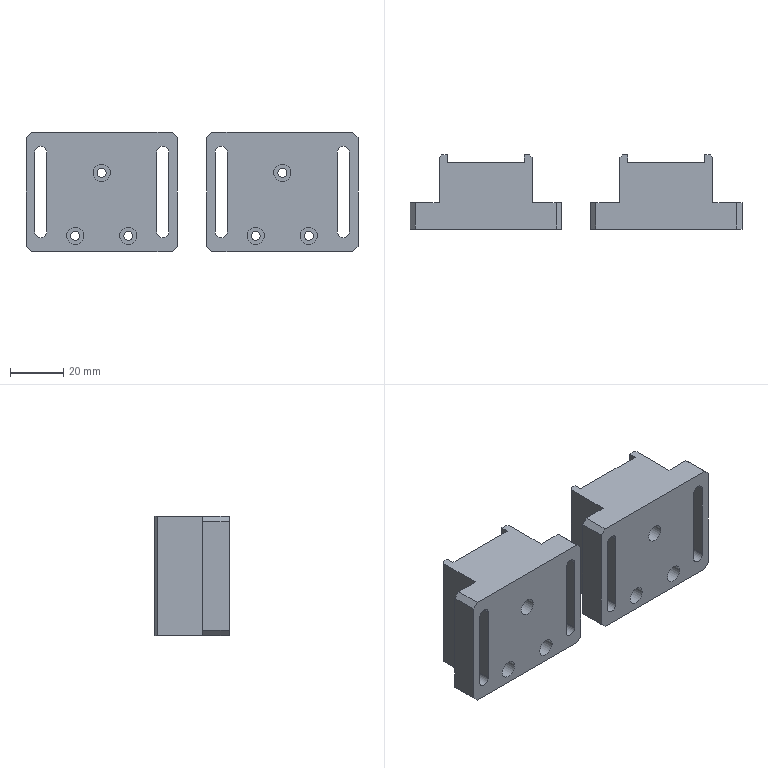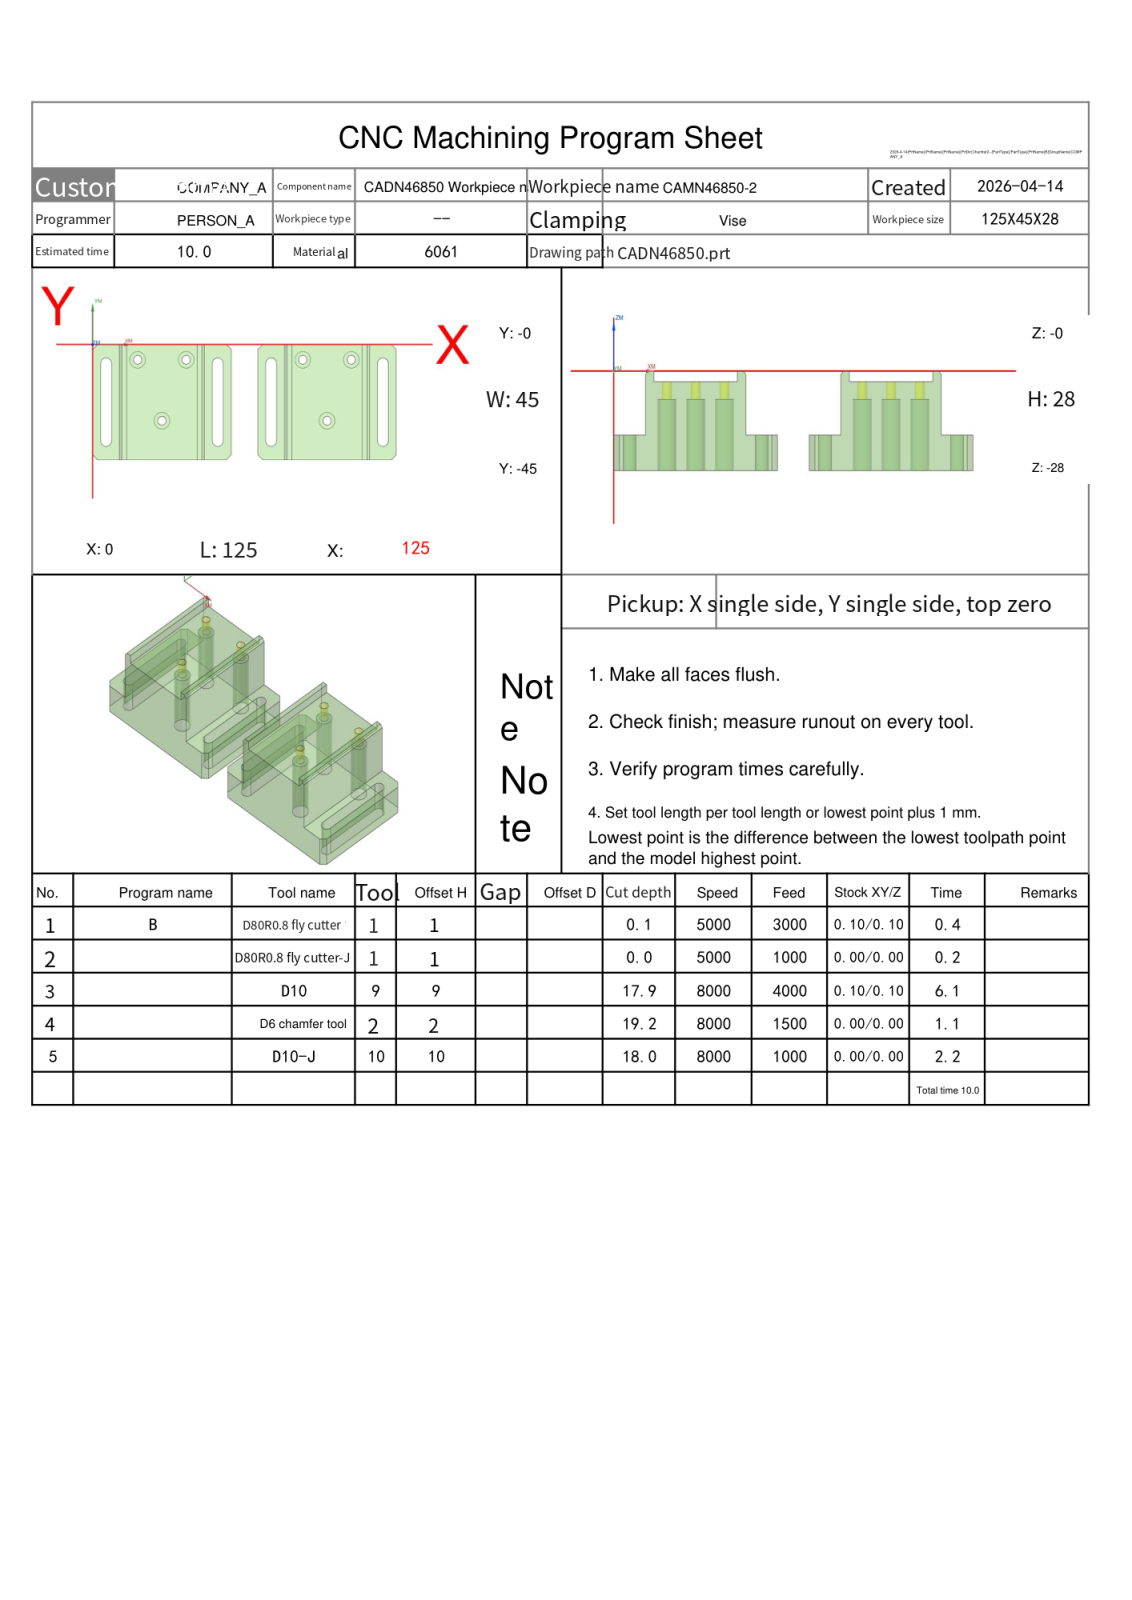NC program | NX | posted by the shop | part box 125 x 28 x 45 mm
Lines 1 to 3146 of 3399, first 2488 of 3144 lines:
%
O0001
(Machine time: 10.92 MIN)
(===Total Tool:4===)
(T1=D80R0.8 fly cutter D=80.  R=0.8  D-  H01 Z=-0.   )
(T9=D10     D=10.  R=0.   D-  H09 Z=-17.9 )
(T2=D6 chamfer tool   D=6.   R=0.   D-  H02 Z=-19.2 )
(T10=D10-J  D=10.  R=0.   D10 H10 Z=-18.  )
G80 G90 G17 G49 G40
G91 G28 Z0
M01
N1 T01 M06
(D80R0.8 fly cutter  D=80. R=0.8 H=01 ce=0.10 di=0.10)
G00 G90 G54 X177.097 Y-22.5 M03 S5000
G43 H01 Z20.
M08
Z3.525
G01 Z1.525 F3000.
X165.097
X-40.097
X-52.097
Z3.525
G00 X177.097
Z3.05
G01 Z1.05
X165.097
X-40.097
X-52.097
Z3.05
G00 X177.097
Z2.575
G01 Z.575
X165.097
X-40.097
X-52.097
Z2.575
G00 X177.097
Z2.1
G01 Z.1
X165.097
X-40.097
X-52.097
Z2.1
G00 Z20.
G91 G28 Z0.0
M05
M09
G91 G28 Z0.0
M01
N2 T01 M06
(D80R0.8 fly cutter-J  D=80. R=0.8 H=01 ce=0.00 di=0.00)
G00 G90 G54 X176.999 Y-22.5 M03 S5000
G43 H01 Z20.
M08
Z2.
G01 Z0.0 F1000.
X164.999
X-39.999
X-51.999
Z2.
G00 Z20.
G91 G28 Z0.0
M05
M09
G91 G28 Z0.0
M01
N3 T09 M06
(D10  D=10. R=0. H=09 ce=0.10 di=0.10)
G00 G90 G54 X133. Y-22.5 M03 S8000
G43 H09 Z11.8
M08
Z.903
G01 Z-.597 F4000.
X129.9
Y-45.03
X125.03 Y-49.9
X119.1
Y4.9
X125.03
X129.9 Y.03
Y-19.836
G02 X129.607 Y-20.543 I-1. J0.0
G01 X125.693 Y-24.457
G03 X125.4 Y-25.164 I.707 J-.707
G01 Y-42.795
G02 X124.5 Y-43.693 I-.9 J.002
X123.6 Y-42.794 I0.0 J.9
G01 Y-2.206
G02 X124.5 Y-1.307 I.9 J-.002
X125.4 Y-2.205 I0.0 J-.9
G01 Y-22.5
Y-23.
X133.
Z.903
G00 Y-22.5
Z.307
G01 Z-1.193
X129.9
Y-45.03
X125.03 Y-49.9
X119.1
Y4.9
X125.03
X129.9 Y.03
Y-19.836
G02 X129.607 Y-20.543 I-1. J0.0
G01 X125.693 Y-24.457
G03 X125.4 Y-25.164 I.707 J-.707
G01 Y-42.795
G02 X124.5 Y-43.693 I-.9 J.002
X123.6 Y-42.794 I0.0 J.9
G01 Y-2.206
G02 X124.5 Y-1.307 I.9 J-.002
X125.4 Y-2.205 I0.0 J-.9
G01 Y-22.5
Y-23.
X133.
Z.307
G00 Y-22.5
Z-.29
G01 Z-1.79
X129.9
Y-45.03
X125.03 Y-49.9
X119.1
Y4.9
X125.03
X129.9 Y.03
Y-19.836
G02 X129.607 Y-20.543 I-1. J0.0
G01 X125.693 Y-24.457
G03 X125.4 Y-25.164 I.707 J-.707
G01 Y-42.795
G02 X124.5 Y-43.693 I-.9 J.002
X123.6 Y-42.794 I0.0 J.9
G01 Y-2.206
G02 X124.5 Y-1.307 I.9 J-.002
X125.4 Y-2.205 I0.0 J-.9
G01 Y-22.5
Y-23.
X133.
Z-.29
G00 Y-22.5
Z-.887
G01 Z-2.387
X129.9
Y-45.03
X125.03 Y-49.9
X119.1
Y4.9
X125.03
X129.9 Y.03
Y-19.836
G02 X129.607 Y-20.543 I-1. J0.0
G01 X125.693 Y-24.457
G03 X125.4 Y-25.164 I.707 J-.707
G01 Y-42.795
G02 X124.5 Y-43.693 I-.9 J.002
X123.6 Y-42.794 I0.0 J.9
G01 Y-2.206
G02 X124.5 Y-1.307 I.9 J-.002
X125.4 Y-2.205 I0.0 J-.9
G01 Y-22.5
Y-23.
X133.
Z-.887
G00 Y-22.5
Z-1.483
G01 Z-2.983
X129.9
Y-45.03
X125.03 Y-49.9
X119.1
Y4.9
X125.03
X129.9 Y.03
Y-19.836
G02 X129.607 Y-20.543 I-1. J0.0
G01 X125.693 Y-24.457
G03 X125.4 Y-25.164 I.707 J-.707
G01 Y-42.795
G02 X124.5 Y-43.693 I-.9 J.002
X123.6 Y-42.794 I0.0 J.9
G01 Y-2.206
G02 X124.5 Y-1.307 I.9 J-.002
X125.4 Y-2.205 I0.0 J-.9
G01 Y-22.5
Y-23.
X133.
Z-1.483
G00 Y-22.5
Z-2.08
G01 Z-3.58
X129.9
Y-45.03
X125.03 Y-49.9
X119.1
Y4.9
X125.03
X129.9 Y.03
Y-19.836
G02 X129.607 Y-20.543 I-1. J0.0
G01 X125.693 Y-24.457
G03 X125.4 Y-25.164 I.707 J-.707
G01 Y-42.795
G02 X124.5 Y-43.693 I-.9 J.002
X123.6 Y-42.794 I0.0 J.9
G01 Y-2.206
G02 X124.5 Y-1.307 I.9 J-.002
X125.4 Y-2.205 I0.0 J-.9
G01 Y-22.5
Y-23.
X133.
Z-2.08
G00 Y-22.5
Z-2.677
G01 Z-4.177
X129.9
Y-45.03
X125.03 Y-49.9
X119.1
Y4.9
X125.03
X129.9 Y.03
Y-19.836
G02 X129.607 Y-20.543 I-1. J0.0
G01 X125.693 Y-24.457
G03 X125.4 Y-25.164 I.707 J-.707
G01 Y-42.795
G02 X124.5 Y-43.693 I-.9 J.002
X123.6 Y-42.794 I0.0 J.9
G01 Y-2.206
G02 X124.5 Y-1.307 I.9 J-.002
X125.4 Y-2.205 I0.0 J-.9
G01 Y-22.5
Y-23.
X133.
Z-2.677
G00 Y-22.5
Z-3.273
G01 Z-4.773
X129.9
Y-45.03
X125.03 Y-49.9
X119.1
Y4.9
X125.03
X129.9 Y.03
Y-19.836
G02 X129.607 Y-20.543 I-1. J0.0
G01 X125.693 Y-24.457
G03 X125.4 Y-25.164 I.707 J-.707
G01 Y-42.795
G02 X124.5 Y-43.693 I-.9 J.002
X123.6 Y-42.794 I0.0 J.9
G01 Y-2.206
G02 X124.5 Y-1.307 I.9 J-.002
X125.4 Y-2.205 I0.0 J-.9
G01 Y-22.5
Y-23.
X133.
Z-3.273
G00 Y-22.5
Z-3.87
G01 Z-5.37
X129.9
Y-45.03
X125.03 Y-49.9
X119.1
Y4.9
X125.03
X129.9 Y.03
Y-19.836
G02 X129.607 Y-20.543 I-1. J0.0
G01 X125.693 Y-24.457
G03 X125.4 Y-25.164 I.707 J-.707
G01 Y-42.795
G02 X124.5 Y-43.693 I-.9 J.002
X123.6 Y-42.794 I0.0 J.9
G01 Y-2.206
G02 X124.5 Y-1.307 I.9 J-.002
X125.4 Y-2.205 I0.0 J-.9
G01 Y-22.5
Y-23.
X133.
Z-3.87
G00 Y-22.5
Z-4.467
G01 Z-5.967
X129.9
Y-45.03
X125.03 Y-49.9
X119.1
Y4.9
X125.03
X129.9 Y.03
Y-19.836
G02 X129.607 Y-20.543 I-1. J0.0
G01 X125.693 Y-24.457
G03 X125.4 Y-25.164 I.707 J-.707
G01 Y-42.795
G02 X124.5 Y-43.693 I-.9 J.002
X123.6 Y-42.794 I0.0 J.9
G01 Y-2.206
G02 X124.5 Y-1.307 I.9 J-.002
X125.4 Y-2.205 I0.0 J-.9
G01 Y-22.5
Y-23.
X133.
Z-4.467
G00 Y-22.5
Z-5.063
G01 Z-6.563
X129.9
Y-45.03
X125.03 Y-49.9
X119.1
Y4.9
X125.03
X129.9 Y.03
Y-19.836
G02 X129.607 Y-20.543 I-1. J0.0
G01 X125.693 Y-24.457
G03 X125.4 Y-25.164 I.707 J-.707
G01 Y-42.795
G02 X124.5 Y-43.693 I-.9 J.002
X123.6 Y-42.794 I0.0 J.9
G01 Y-2.206
G02 X124.5 Y-1.307 I.9 J-.002
X125.4 Y-2.205 I0.0 J-.9
G01 Y-22.5
Y-23.
X133.
Z-5.063
G00 Y-22.5
Z-5.66
G01 Z-7.16
X129.9
Y-45.03
X125.03 Y-49.9
X119.1
Y4.9
X125.03
X129.9 Y.03
Y-19.836
G02 X129.607 Y-20.543 I-1. J0.0
G01 X125.693 Y-24.457
G03 X125.4 Y-25.164 I.707 J-.707
G01 Y-42.795
G02 X124.5 Y-43.693 I-.9 J.002
X123.6 Y-42.794 I0.0 J.9
G01 Y-2.206
G02 X124.5 Y-1.307 I.9 J-.002
X125.4 Y-2.205 I0.0 J-.9
G01 Y-22.5
Y-23.
X133.
Z-5.66
G00 Y-22.5
Z-6.257
G01 Z-7.757
X129.9
Y-45.03
X125.03 Y-49.9
X119.1
Y4.9
X125.03
X129.9 Y.03
Y-19.836
G02 X129.607 Y-20.543 I-1. J0.0
G01 X125.693 Y-24.457
G03 X125.4 Y-25.164 I.707 J-.707
G01 Y-42.795
G02 X124.5 Y-43.693 I-.9 J.002
X123.6 Y-42.794 I0.0 J.9
G01 Y-2.206
G02 X124.5 Y-1.307 I.9 J-.002
X125.4 Y-2.205 I0.0 J-.9
G01 Y-22.5
Y-23.
X133.
Z-6.257
G00 Y-22.5
Z-6.853
G01 Z-8.353
X129.9
Y-45.03
X125.03 Y-49.9
X119.1
Y4.9
X125.03
X129.9 Y.03
Y-19.836
G02 X129.607 Y-20.543 I-1. J0.0
G01 X125.693 Y-24.457
G03 X125.4 Y-25.164 I.707 J-.707
G01 Y-42.795
G02 X124.5 Y-43.693 I-.9 J.002
X123.6 Y-42.794 I0.0 J.9
G01 Y-2.206
G02 X124.5 Y-1.307 I.9 J-.002
X125.4 Y-2.205 I0.0 J-.9
G01 Y-22.5
Y-23.
X133.
Z-6.853
G00 Y-22.5
Z-7.45
G01 Z-8.95
X129.9
Y-45.03
X125.03 Y-49.9
X119.1
Y4.9
X125.03
X129.9 Y.03
Y-19.836
G02 X129.607 Y-20.543 I-1. J0.0
G01 X125.693 Y-24.457
G03 X125.4 Y-25.164 I.707 J-.707
G01 Y-42.795
G02 X124.5 Y-43.693 I-.9 J.002
X123.6 Y-42.794 I0.0 J.9
G01 Y-2.206
G02 X124.5 Y-1.307 I.9 J-.002
X125.4 Y-2.205 I0.0 J-.9
G01 Y-22.5
Y-23.
X133.
Z-7.45
G00 Y-22.5
Z-8.047
G01 Z-9.547
X129.9
Y-45.03
X125.03 Y-49.9
X119.1
Y4.9
X125.03
X129.9 Y.03
Y-19.836
G02 X129.607 Y-20.543 I-1. J0.0
G01 X125.693 Y-24.457
G03 X125.4 Y-25.164 I.707 J-.707
G01 Y-42.795
G02 X124.5 Y-43.693 I-.9 J.002
X123.6 Y-42.794 I0.0 J.9
G01 Y-2.206
G02 X124.5 Y-1.307 I.9 J-.002
X125.4 Y-2.205 I0.0 J-.9
G01 Y-22.5
Y-23.
X133.
Z-8.047
G00 Y-22.5
Z-8.643
G01 Z-10.143
X129.9
Y-45.03
X125.03 Y-49.9
X119.1
Y4.9
X125.03
X129.9 Y.03
Y-19.836
G02 X129.607 Y-20.543 I-1. J0.0
G01 X125.693 Y-24.457
G03 X125.4 Y-25.164 I.707 J-.707
G01 Y-42.795
G02 X124.5 Y-43.693 I-.9 J.002
X123.6 Y-42.794 I0.0 J.9
G01 Y-2.206
G02 X124.5 Y-1.307 I.9 J-.002
X125.4 Y-2.205 I0.0 J-.9
G01 Y-22.5
Y-23.
X133.
Z-8.643
G00 Y-22.5
Z-9.24
G01 Z-10.74
X129.9
Y-45.03
X125.03 Y-49.9
X119.1
Y4.9
X125.03
X129.9 Y.03
Y-19.836
G02 X129.607 Y-20.543 I-1. J0.0
G01 X125.693 Y-24.457
G03 X125.4 Y-25.164 I.707 J-.707
G01 Y-42.795
G02 X124.5 Y-43.693 I-.9 J.002
X123.6 Y-42.794 I0.0 J.9
G01 Y-2.206
G02 X124.5 Y-1.307 I.9 J-.002
X125.4 Y-2.205 I0.0 J-.9
G01 Y-22.5
Y-23.
X133.
Z-9.24
G00 Y-22.5
Z-9.837
G01 Z-11.337
X129.9
Y-45.03
X125.03 Y-49.9
X119.1
Y4.9
X125.03
X129.9 Y.03
Y-19.836
G02 X129.607 Y-20.543 I-1. J0.0
G01 X125.693 Y-24.457
G03 X125.4 Y-25.164 I.707 J-.707
G01 Y-42.795
G02 X124.5 Y-43.693 I-.9 J.002
X123.6 Y-42.794 I0.0 J.9
G01 Y-2.206
G02 X124.5 Y-1.307 I.9 J-.002
X125.4 Y-2.205 I0.0 J-.9
G01 Y-22.5
Y-23.
X133.
Z-9.837
G00 Y-22.5
Z-10.433
G01 Z-11.933
X129.9
Y-45.03
X125.03 Y-49.9
X119.1
Y4.9
X125.03
X129.9 Y.03
Y-19.836
G02 X129.607 Y-20.543 I-1. J0.0
G01 X125.693 Y-24.457
G03 X125.4 Y-25.164 I.707 J-.707
G01 Y-42.795
G02 X124.5 Y-43.693 I-.9 J.002
X123.6 Y-42.794 I0.0 J.9
G01 Y-2.206
G02 X124.5 Y-1.307 I.9 J-.002
X125.4 Y-2.205 I0.0 J-.9
G01 Y-22.5
Y-23.
X133.
Z-10.433
G00 Y-22.5
Z-11.03
G01 Z-12.53
X129.9
Y-45.03
X125.03 Y-49.9
X119.1
Y4.9
X125.03
X129.9 Y.03
Y-19.836
G02 X129.607 Y-20.543 I-1. J0.0
G01 X125.693 Y-24.457
G03 X125.4 Y-25.164 I.707 J-.707
G01 Y-42.795
G02 X124.5 Y-43.693 I-.9 J.002
X123.6 Y-42.794 I0.0 J.9
G01 Y-2.206
G02 X124.5 Y-1.307 I.9 J-.002
X125.4 Y-2.205 I0.0 J-.9
G01 Y-22.5
Y-23.
X133.
Z-11.03
G00 Y-22.5
Z-11.627
G01 Z-13.127
X129.9
Y-45.03
X125.03 Y-49.9
X119.1
Y4.9
X125.03
X129.9 Y.03
Y-19.836
G02 X129.607 Y-20.543 I-1. J0.0
G01 X125.693 Y-24.457
G03 X125.4 Y-25.164 I.707 J-.707
G01 Y-42.795
G02 X124.5 Y-43.693 I-.9 J.002
X123.6 Y-42.794 I0.0 J.9
G01 Y-2.206
G02 X124.5 Y-1.307 I.9 J-.002
X125.4 Y-2.205 I0.0 J-.9
G01 Y-22.5
Y-23.
X133.
Z-11.627
G00 Y-22.5
Z-12.223
G01 Z-13.723
X129.9
Y-45.03
X125.03 Y-49.9
X119.1
Y4.9
X125.03
X129.9 Y.03
Y-19.836
G02 X129.607 Y-20.543 I-1. J0.0
G01 X125.693 Y-24.457
G03 X125.4 Y-25.164 I.707 J-.707
G01 Y-42.795
G02 X124.5 Y-43.693 I-.9 J.002
X123.6 Y-42.794 I0.0 J.9
G01 Y-2.206
G02 X124.5 Y-1.307 I.9 J-.002
X125.4 Y-2.205 I0.0 J-.9
G01 Y-22.5
Y-23.
X133.
Z-12.223
G00 Y-22.5
Z-12.82
G01 Z-14.32
X129.9
Y-45.03
X125.03 Y-49.9
X119.1
Y4.9
X125.03
X129.9 Y.03
Y-19.836
G02 X129.607 Y-20.543 I-1. J0.0
G01 X125.693 Y-24.457
G03 X125.4 Y-25.164 I.707 J-.707
G01 Y-42.795
G02 X124.5 Y-43.693 I-.9 J.002
X123.6 Y-42.794 I0.0 J.9
G01 Y-2.206
G02 X124.5 Y-1.307 I.9 J-.002
X125.4 Y-2.205 I0.0 J-.9
G01 Y-22.5
Y-23.
X133.
Z-12.82
G00 Y-22.5
Z-13.417
G01 Z-14.917
X129.9
Y-45.03
X125.03 Y-49.9
X119.1
Y4.9
X125.03
X129.9 Y.03
Y-19.836
G02 X129.607 Y-20.543 I-1. J0.0
G01 X125.693 Y-24.457
G03 X125.4 Y-25.164 I.707 J-.707
G01 Y-42.795
G02 X124.5 Y-43.693 I-.9 J.002
X123.6 Y-42.794 I0.0 J.9
G01 Y-2.206
G02 X124.5 Y-1.307 I.9 J-.002
X125.4 Y-2.205 I0.0 J-.9
G01 Y-22.5
Y-23.
X133.
Z-13.417
G00 Y-22.5
Z-14.013
G01 Z-15.513
X129.9
Y-45.03
X125.03 Y-49.9
X119.1
Y4.9
X125.03
X129.9 Y.03
Y-19.836
G02 X129.607 Y-20.543 I-1. J0.0
G01 X125.693 Y-24.457
G03 X125.4 Y-25.164 I.707 J-.707
G01 Y-42.795
G02 X124.5 Y-43.693 I-.9 J.002
X123.6 Y-42.794 I0.0 J.9
G01 Y-2.206
G02 X124.5 Y-1.307 I.9 J-.002
X125.4 Y-2.205 I0.0 J-.9
G01 Y-22.5
Y-23.
X133.
Z-14.013
G00 Y-22.5
Z-14.61
G01 Z-16.11
X129.9
Y-45.03
X125.03 Y-49.9
X119.1
Y4.9
X125.03
X129.9 Y.03
Y-19.836
G02 X129.607 Y-20.543 I-1. J0.0
G01 X125.693 Y-24.457
G03 X125.4 Y-25.164 I.707 J-.707
G01 Y-42.795
G02 X124.5 Y-43.693 I-.9 J.002
X123.6 Y-42.794 I0.0 J.9
G01 Y-2.206
G02 X124.5 Y-1.307 I.9 J-.002
X125.4 Y-2.205 I0.0 J-.9
G01 Y-22.5
Y-23.
X133.
Z-14.61
G00 Y-22.5
Z-15.207
G01 Z-16.707
X129.9
Y-45.03
X125.03 Y-49.9
X119.1
Y4.9
X125.03
X129.9 Y.03
Y-19.836
G02 X129.607 Y-20.543 I-1. J0.0
G01 X125.693 Y-24.457
G03 X125.4 Y-25.164 I.707 J-.707
G01 Y-42.795
G02 X124.5 Y-43.693 I-.9 J.002
X123.6 Y-42.794 I0.0 J.9
G01 Y-2.206
G02 X124.5 Y-1.307 I.9 J-.002
X125.4 Y-2.205 I0.0 J-.9
G01 Y-22.5
Y-23.
X133.
Z-15.207
G00 Y-22.5
Z-15.803
G01 Z-17.303
X129.9
Y-45.03
X125.03 Y-49.9
X119.1
Y4.9
X125.03
X129.9 Y.03
Y-19.836
G02 X129.607 Y-20.543 I-1. J0.0
G01 X125.693 Y-24.457
G03 X125.4 Y-25.164 I.707 J-.707
G01 Y-42.795
G02 X124.5 Y-43.693 I-.9 J.002
X123.6 Y-42.794 I0.0 J.9
G01 Y-2.206
G02 X124.5 Y-1.307 I.9 J-.002
X125.4 Y-2.205 I0.0 J-.9
G01 Y-22.5
Y-23.
X133.
Z-15.803
G00 Y-22.5
Z-16.4
G01 Z-17.9
X129.9
Y-45.03
X125.03 Y-49.9
X119.1
Y4.9
X125.03
X129.9 Y.03
Y-19.836
G02 X129.607 Y-20.543 I-1. J0.0
G01 X125.693 Y-24.457
G03 X125.4 Y-25.164 I.707 J-.707
G01 Y-42.795
G02 X124.5 Y-43.693 I-.9 J.002
X123.6 Y-42.794 I0.0 J.9
G01 Y-2.206
G02 X124.5 Y-1.307 I.9 J-.002
X125.4 Y-2.205 I0.0 J-.9
G01 Y-22.5
Y-23.
X133.
Z-16.4
G00 Z11.8
X62.5 Y-52.57
Z.903
G01 Z-.597
Y-49.47
X57.46
X57.03 Y-49.9
X51.1
Y4.9
X57.03
X57.46 Y4.47
X67.54
X67.97 Y4.9
X73.9
Y-49.9
X67.97
X67.54 Y-49.47
X65.535
G02 X64.703 Y-49.025 I0.0 J1.
G01 X60.293 Y-42.41
G03 X59.531 Y-41.967 I-.832 J-.555
G02 X58.6 Y-40.972 I.069 J.998
G01 Y-4.028
G02 X59.598 Y-3.03 I1. J-.002
G01 X65.402
G02 X66.4 Y-4.028 I-.002 J-1.
G01 Y-40.972
G02 X65.402 Y-41.97 I-1. J.002
G01 X62.5
X62.
Y-52.57
Z.903
G00 X62.5
Z.307
G01 Z-1.193
Y-49.47
X57.46
X57.03 Y-49.9
X51.1
Y4.9
X57.03
X57.46 Y4.47
X67.54
X67.97 Y4.9
X73.9
Y-49.9
X67.97
X67.54 Y-49.47
X65.535
G02 X64.703 Y-49.025 I0.0 J1.
G01 X60.293 Y-42.41
G03 X59.531 Y-41.967 I-.832 J-.555
G02 X58.6 Y-40.972 I.069 J.998
G01 Y-4.028
G02 X59.598 Y-3.03 I1. J-.002
G01 X65.402
G02 X66.4 Y-4.028 I-.002 J-1.
G01 Y-40.972
G02 X65.402 Y-41.97 I-1. J.002
G01 X62.5
X62.
Y-52.57
Z.307
G00 X62.5
Z-.29
G01 Z-1.79
Y-49.47
X57.46
X57.03 Y-49.9
X51.1
Y4.9
X57.03
X57.46 Y4.47
X67.54
X67.97 Y4.9
X73.9
Y-49.9
X67.97
X67.54 Y-49.47
X65.535
G02 X64.703 Y-49.025 I0.0 J1.
G01 X60.293 Y-42.41
G03 X59.531 Y-41.967 I-.832 J-.555
G02 X58.6 Y-40.972 I.069 J.998
G01 Y-4.028
G02 X59.598 Y-3.03 I1. J-.002
G01 X65.402
G02 X66.4 Y-4.028 I-.002 J-1.
G01 Y-40.972
G02 X65.402 Y-41.97 I-1. J.002
G01 X62.5
X62.
Y-52.57
Z-.29
G00 X62.5
Z-.887
G01 Z-2.387
Y-49.47
X57.46
X57.03 Y-49.9
X51.1
Y4.9
X57.03
X57.46 Y4.47
X67.54
X67.97 Y4.9
X73.9
Y-49.9
X67.97
X67.54 Y-49.47
X65.535
G02 X64.703 Y-49.025 I0.0 J1.
G01 X60.293 Y-42.41
G03 X59.531 Y-41.967 I-.832 J-.555
G02 X58.6 Y-40.972 I.069 J.998
G01 Y-4.028
G02 X59.598 Y-3.03 I1. J-.002
G01 X65.402
G02 X66.4 Y-4.028 I-.002 J-1.
G01 Y-40.972
G02 X65.402 Y-41.97 I-1. J.002
G01 X62.5
X62.
Y-52.57
Z-.887
G00 X62.5
Z-1.483
G01 Z-2.983
Y-49.47
X57.46
X57.03 Y-49.9
X51.1
Y4.9
X57.03
X57.46 Y4.47
X67.54
X67.97 Y4.9
X73.9
Y-49.9
X67.97
X67.54 Y-49.47
X65.535
G02 X64.703 Y-49.025 I0.0 J1.
G01 X60.293 Y-42.41
G03 X59.531 Y-41.967 I-.832 J-.555
G02 X58.6 Y-40.972 I.069 J.998
G01 Y-4.028
G02 X59.598 Y-3.03 I1. J-.002
G01 X65.402
G02 X66.4 Y-4.028 I-.002 J-1.
G01 Y-40.972
G02 X65.402 Y-41.97 I-1. J.002
G01 X62.5
X62.
Y-52.57
Z-1.483
G00 X62.5
Z-2.08
G01 Z-3.58
Y-49.47
X57.46
X57.03 Y-49.9
X51.1
Y4.9
X57.03
X57.46 Y4.47
X67.54
X67.97 Y4.9
X73.9
Y-49.9
X67.97
X67.54 Y-49.47
X65.535
G02 X64.703 Y-49.025 I0.0 J1.
G01 X60.293 Y-42.41
G03 X59.531 Y-41.967 I-.832 J-.555
G02 X58.6 Y-40.972 I.069 J.998
G01 Y-4.028
G02 X59.598 Y-3.03 I1. J-.002
G01 X65.402
G02 X66.4 Y-4.028 I-.002 J-1.
G01 Y-40.972
G02 X65.402 Y-41.97 I-1. J.002
G01 X62.5
X62.
Y-52.57
Z-2.08
G00 X62.5
Z-2.677
G01 Z-4.177
Y-49.47
X57.46
X57.03 Y-49.9
X51.1
Y4.9
X57.03
X57.46 Y4.47
X67.54
X67.97 Y4.9
X73.9
Y-49.9
X67.97
X67.54 Y-49.47
X65.535
G02 X64.703 Y-49.025 I0.0 J1.
G01 X60.293 Y-42.41
G03 X59.531 Y-41.967 I-.832 J-.555
G02 X58.6 Y-40.972 I.069 J.998
G01 Y-4.028
G02 X59.598 Y-3.03 I1. J-.002
G01 X65.402
G02 X66.4 Y-4.028 I-.002 J-1.
G01 Y-40.972
G02 X65.402 Y-41.97 I-1. J.002
G01 X62.5
X62.
Y-52.57
Z-2.677
G00 X62.5
Z-3.273
G01 Z-4.773
Y-49.47
X57.46
X57.03 Y-49.9
X51.1
Y4.9
X57.03
X57.46 Y4.47
X67.54
X67.97 Y4.9
X73.9
Y-49.9
X67.97
X67.54 Y-49.47
X65.535
G02 X64.703 Y-49.025 I0.0 J1.
G01 X60.293 Y-42.41
G03 X59.531 Y-41.967 I-.832 J-.555
G02 X58.6 Y-40.972 I.069 J.998
G01 Y-4.028
G02 X59.598 Y-3.03 I1. J-.002
G01 X65.402
G02 X66.4 Y-4.028 I-.002 J-1.
G01 Y-40.972
G02 X65.402 Y-41.97 I-1. J.002
G01 X62.5
X62.
Y-52.57
Z-3.273
G00 X62.5
Z-3.87
G01 Z-5.37
Y-49.47
X57.46
X57.03 Y-49.9
X51.1
Y4.9
X57.03
X57.46 Y4.47
X67.54
X67.97 Y4.9
X73.9
Y-49.9
X67.97
X67.54 Y-49.47
X65.535
G02 X64.703 Y-49.025 I0.0 J1.
G01 X60.293 Y-42.41
G03 X59.531 Y-41.967 I-.832 J-.555
G02 X58.6 Y-40.972 I.069 J.998
G01 Y-4.028
G02 X59.598 Y-3.03 I1. J-.002
G01 X65.402
G02 X66.4 Y-4.028 I-.002 J-1.
G01 Y-40.972
G02 X65.402 Y-41.97 I-1. J.002
G01 X62.5
X62.
Y-52.57
Z-3.87
G00 X62.5
Z-4.467
G01 Z-5.967
Y-49.47
X57.46
X57.03 Y-49.9
X51.1
Y4.9
X57.03
X57.46 Y4.47
X67.54
X67.97 Y4.9
X73.9
Y-49.9
X67.97
X67.54 Y-49.47
X65.535
G02 X64.703 Y-49.025 I0.0 J1.
G01 X60.293 Y-42.41
G03 X59.531 Y-41.967 I-.832 J-.555
G02 X58.6 Y-40.972 I.069 J.998
G01 Y-4.028
G02 X59.598 Y-3.03 I1. J-.002
G01 X65.402
G02 X66.4 Y-4.028 I-.002 J-1.
G01 Y-40.972
G02 X65.402 Y-41.97 I-1. J.002
G01 X62.5
X62.
Y-52.57
Z-4.467
G00 X62.5
Z-5.063
G01 Z-6.563
Y-49.47
X57.46
X57.03 Y-49.9
X51.1
Y4.9
X57.03
X57.46 Y4.47
X67.54
X67.97 Y4.9
X73.9
Y-49.9
X67.97
X67.54 Y-49.47
X65.535
G02 X64.703 Y-49.025 I0.0 J1.
G01 X60.293 Y-42.41
G03 X59.531 Y-41.967 I-.832 J-.555
G02 X58.6 Y-40.972 I.069 J.998
G01 Y-4.028
G02 X59.598 Y-3.03 I1. J-.002
G01 X65.402
G02 X66.4 Y-4.028 I-.002 J-1.
G01 Y-40.972
G02 X65.402 Y-41.97 I-1. J.002
G01 X62.5
X62.
Y-52.57
Z-5.063
G00 X62.5
Z-5.66
G01 Z-7.16
Y-49.47
X57.46
X57.03 Y-49.9
X51.1
Y4.9
X57.03
X57.46 Y4.47
X67.54
X67.97 Y4.9
X73.9
Y-49.9
X67.97
X67.54 Y-49.47
X65.535
G02 X64.703 Y-49.025 I0.0 J1.
G01 X60.293 Y-42.41
G03 X59.531 Y-41.967 I-.832 J-.555
G02 X58.6 Y-40.972 I.069 J.998
G01 Y-4.028
G02 X59.598 Y-3.03 I1. J-.002
G01 X65.402
G02 X66.4 Y-4.028 I-.002 J-1.
G01 Y-40.972
G02 X65.402 Y-41.97 I-1. J.002
G01 X62.5
X62.
Y-52.57
Z-5.66
G00 X62.5
Z-6.257
G01 Z-7.757
Y-49.47
X57.46
X57.03 Y-49.9
X51.1
Y4.9
X57.03
X57.46 Y4.47
X67.54
X67.97 Y4.9
X73.9
Y-49.9
X67.97
X67.54 Y-49.47
X65.535
G02 X64.703 Y-49.025 I0.0 J1.
G01 X60.293 Y-42.41
G03 X59.531 Y-41.967 I-.832 J-.555
G02 X58.6 Y-40.972 I.069 J.998
G01 Y-4.028
G02 X59.598 Y-3.03 I1. J-.002
G01 X65.402
G02 X66.4 Y-4.028 I-.002 J-1.
G01 Y-40.972
G02 X65.402 Y-41.97 I-1. J.002
G01 X62.5
X62.
Y-52.57
Z-6.257
G00 X62.5
Z-6.853
G01 Z-8.353
Y-49.47
X57.46
X57.03 Y-49.9
X51.1
Y4.9
X57.03
X57.46 Y4.47
X67.54
X67.97 Y4.9
X73.9
Y-49.9
X67.97
X67.54 Y-49.47
X65.535
G02 X64.703 Y-49.025 I0.0 J1.
G01 X60.293 Y-42.41
G03 X59.531 Y-41.967 I-.832 J-.555
G02 X58.6 Y-40.972 I.069 J.998
G01 Y-4.028
G02 X59.598 Y-3.03 I1. J-.002
G01 X65.402
G02 X66.4 Y-4.028 I-.002 J-1.
G01 Y-40.972
G02 X65.402 Y-41.97 I-1. J.002
G01 X62.5
X62.
Y-52.57
Z-6.853
G00 X62.5
Z-7.45
G01 Z-8.95
Y-49.47
X57.46
X57.03 Y-49.9
X51.1
Y4.9
X57.03
X57.46 Y4.47
X67.54
X67.97 Y4.9
X73.9
Y-49.9
X67.97
X67.54 Y-49.47
X65.535
G02 X64.703 Y-49.025 I0.0 J1.
G01 X60.293 Y-42.41
G03 X59.531 Y-41.967 I-.832 J-.555
G02 X58.6 Y-40.972 I.069 J.998
G01 Y-4.028
G02 X59.598 Y-3.03 I1. J-.002
G01 X65.402
G02 X66.4 Y-4.028 I-.002 J-1.
G01 Y-40.972
G02 X65.402 Y-41.97 I-1. J.002
G01 X62.5
X62.
Y-52.57
Z-7.45
G00 X62.5
Z-8.047
G01 Z-9.547
Y-49.47
X57.46
X57.03 Y-49.9
X51.1
Y4.9
X57.03
X57.46 Y4.47
X67.54
X67.97 Y4.9
X73.9
Y-49.9
X67.97
X67.54 Y-49.47
X65.535
G02 X64.703 Y-49.025 I0.0 J1.
G01 X60.293 Y-42.41
G03 X59.531 Y-41.967 I-.832 J-.555
G02 X58.6 Y-40.972 I.069 J.998
G01 Y-4.028
G02 X59.598 Y-3.03 I1. J-.002
G01 X65.402
G02 X66.4 Y-4.028 I-.002 J-1.
G01 Y-40.972
G02 X65.402 Y-41.97 I-1. J.002
G01 X62.5
X62.
Y-52.57
Z-8.047
G00 X62.5
Z-8.643
G01 Z-10.143
Y-49.47
X57.46
X57.03 Y-49.9
X51.1
Y4.9
X57.03
X57.46 Y4.47
X67.54
X67.97 Y4.9
X73.9
Y-49.9
X67.97
X67.54 Y-49.47
X65.535
G02 X64.703 Y-49.025 I0.0 J1.
G01 X60.293 Y-42.41
G03 X59.531 Y-41.967 I-.832 J-.555
G02 X58.6 Y-40.972 I.069 J.998
G01 Y-4.028
G02 X59.598 Y-3.03 I1. J-.002
G01 X65.402
G02 X66.4 Y-4.028 I-.002 J-1.
G01 Y-40.972
G02 X65.402 Y-41.97 I-1. J.002
G01 X62.5
X62.
Y-52.57
Z-8.643
G00 X62.5
Z-9.24
G01 Z-10.74
Y-49.47
X57.46
X57.03 Y-49.9
X51.1
Y4.9
X57.03
X57.46 Y4.47
X67.54
X67.97 Y4.9
X73.9
Y-49.9
X67.97
X67.54 Y-49.47
X65.535
G02 X64.703 Y-49.025 I0.0 J1.
G01 X60.293 Y-42.41
G03 X59.531 Y-41.967 I-.832 J-.555
G02 X58.6 Y-40.972 I.069 J.998
G01 Y-4.028
G02 X59.598 Y-3.03 I1. J-.002
G01 X65.402
G02 X66.4 Y-4.028 I-.002 J-1.
G01 Y-40.972
G02 X65.402 Y-41.97 I-1. J.002
G01 X62.5
X62.
Y-52.57
Z-9.24
G00 X62.5
Z-9.837
G01 Z-11.337
Y-49.47
X57.46
X57.03 Y-49.9
X51.1
Y4.9
X57.03
X57.46 Y4.47
X67.54
X67.97 Y4.9
X73.9
Y-49.9
X67.97
X67.54 Y-49.47
X65.535
G02 X64.703 Y-49.025 I0.0 J1.
G01 X60.293 Y-42.41
G03 X59.531 Y-41.967 I-.832 J-.555
G02 X58.6 Y-40.972 I.069 J.998
G01 Y-4.028
G02 X59.598 Y-3.03 I1. J-.002
G01 X65.402
G02 X66.4 Y-4.028 I-.002 J-1.
G01 Y-40.972
G02 X65.402 Y-41.97 I-1. J.002
G01 X62.5
X62.
Y-52.57
Z-9.837
G00 X62.5
Z-10.433
G01 Z-11.933
Y-49.47
X57.46
X57.03 Y-49.9
X51.1
Y4.9
X57.03
X57.46 Y4.47
X67.54
X67.97 Y4.9
X73.9
Y-49.9
X67.97
X67.54 Y-49.47
X65.535
G02 X64.703 Y-49.025 I0.0 J1.
G01 X60.293 Y-42.41
G03 X59.531 Y-41.967 I-.832 J-.555
G02 X58.6 Y-40.972 I.069 J.998
G01 Y-4.028
G02 X59.598 Y-3.03 I1. J-.002
G01 X65.402
G02 X66.4 Y-4.028 I-.002 J-1.
G01 Y-40.972
G02 X65.402 Y-41.97 I-1. J.002
G01 X62.5
X62.
Y-52.57
Z-10.433
G00 X62.5
Z-11.03
G01 Z-12.53
Y-49.47
X57.46
X57.03 Y-49.9
X51.1
Y4.9
X57.03
X57.46 Y4.47
X67.54
X67.97 Y4.9
X73.9
Y-49.9
X67.97
X67.54 Y-49.47
X65.535
G02 X64.703 Y-49.025 I0.0 J1.
G01 X60.293 Y-42.41
G03 X59.531 Y-41.967 I-.832 J-.555
G02 X58.6 Y-40.972 I.069 J.998
G01 Y-4.028
G02 X59.598 Y-3.03 I1. J-.002
G01 X65.402
G02 X66.4 Y-4.028 I-.002 J-1.
G01 Y-40.972
G02 X65.402 Y-41.97 I-1. J.002
G01 X62.5
X62.
Y-52.57
Z-11.03
G00 X62.5
Z-11.627
G01 Z-13.127
Y-49.47
X57.46
X57.03 Y-49.9
X51.1
Y4.9
X57.03
X57.46 Y4.47
X67.54
X67.97 Y4.9
X73.9
Y-49.9
X67.97
X67.54 Y-49.47
X65.535
G02 X64.703 Y-49.025 I0.0 J1.
G01 X60.293 Y-42.41
G03 X59.531 Y-41.967 I-.832 J-.555
G02 X58.6 Y-40.972 I.069 J.998
G01 Y-4.028
G02 X59.598 Y-3.03 I1. J-.002
G01 X65.402
G02 X66.4 Y-4.028 I-.002 J-1.
G01 Y-40.972
G02 X65.402 Y-41.97 I-1. J.002
G01 X62.5
X62.
Y-52.57
Z-11.627
G00 X62.5
Z-12.223
G01 Z-13.723
Y-49.47
X57.46
X57.03 Y-49.9
X51.1
Y4.9
X57.03
X57.46 Y4.47
X67.54
X67.97 Y4.9
X73.9
Y-49.9
X67.97
X67.54 Y-49.47
X65.535
G02 X64.703 Y-49.025 I0.0 J1.
G01 X60.293 Y-42.41
G03 X59.531 Y-41.967 I-.832 J-.555
G02 X58.6 Y-40.972 I.069 J.998
G01 Y-4.028
G02 X59.598 Y-3.03 I1. J-.002
G01 X65.402
G02 X66.4 Y-4.028 I-.002 J-1.
G01 Y-40.972
G02 X65.402 Y-41.97 I-1. J.002
G01 X62.5
X62.
Y-52.57
Z-12.223
G00 X62.5
Z-12.82
G01 Z-14.32
Y-49.47
X57.46
X57.03 Y-49.9
X51.1
Y4.9
X57.03
X57.46 Y4.47
X67.54
X67.97 Y4.9
X73.9
Y-49.9
X67.97
X67.54 Y-49.47
X65.535
G02 X64.703 Y-49.025 I0.0 J1.
G01 X60.293 Y-42.41
G03 X59.531 Y-41.967 I-.832 J-.555
G02 X58.6 Y-40.972 I.069 J.998
G01 Y-4.028
G02 X59.598 Y-3.03 I1. J-.002
G01 X65.402
G02 X66.4 Y-4.028 I-.002 J-1.
G01 Y-40.972
G02 X65.402 Y-41.97 I-1. J.002
G01 X62.5
X62.
Y-52.57
Z-12.82
G00 X62.5
Z-13.417
G01 Z-14.917
Y-49.47
X57.46
X57.03 Y-49.9
X51.1
Y4.9
X57.03
X57.46 Y4.47
X67.54
X67.97 Y4.9
X73.9
Y-49.9
X67.97
X67.54 Y-49.47
X65.535
G02 X64.703 Y-49.025 I0.0 J1.
G01 X60.293 Y-42.41
G03 X59.531 Y-41.967 I-.832 J-.555
G02 X58.6 Y-40.972 I.069 J.998
G01 Y-4.028
G02 X59.598 Y-3.03 I1. J-.002
G01 X65.402
G02 X66.4 Y-4.028 I-.002 J-1.
G01 Y-40.972
G02 X65.402 Y-41.97 I-1. J.002
G01 X62.5
X62.
Y-52.57
Z-13.417
G00 X62.5
Z-14.013
G01 Z-15.513
Y-49.47
X57.46
X57.03 Y-49.9
X51.1
Y4.9
X57.03
X57.46 Y4.47
X67.54
X67.97 Y4.9
X73.9
Y-49.9
X67.97
X67.54 Y-49.47
X65.535
G02 X64.703 Y-49.025 I0.0 J1.
G01 X60.293 Y-42.41
G03 X59.531 Y-41.967 I-.832 J-.555
G02 X58.6 Y-40.972 I.069 J.998
G01 Y-4.028
G02 X59.598 Y-3.03 I1. J-.002
G01 X65.402
G02 X66.4 Y-4.028 I-.002 J-1.
G01 Y-40.972
G02 X65.402 Y-41.97 I-1. J.002
G01 X62.5
X62.
Y-52.57
Z-14.013
G00 X62.5
Z-14.61
G01 Z-16.11
Y-49.47
X57.46
X57.03 Y-49.9
X51.1
Y4.9
X57.03
X57.46 Y4.47
X67.54
X67.97 Y4.9
X73.9
Y-49.9
X67.97
X67.54 Y-49.47
X65.535
G02 X64.703 Y-49.025 I0.0 J1.
G01 X60.293 Y-42.41
G03 X59.531 Y-41.967 I-.832 J-.555
G02 X58.6 Y-40.972 I.069 J.998
G01 Y-4.028
G02 X59.598 Y-3.03 I1. J-.002
G01 X65.402
G02 X66.4 Y-4.028 I-.002 J-1.
G01 Y-40.972
G02 X65.402 Y-41.97 I-1. J.002
G01 X62.5
X62.
Y-52.57
Z-14.61
G00 X62.5
Z-15.207
G01 Z-16.707
Y-49.47
X57.46
X57.03 Y-49.9
X51.1
Y4.9
X57.03
X57.46 Y4.47
X67.54
X67.97 Y4.9
X73.9
Y-49.9
X67.97
X67.54 Y-49.47
X65.535
G02 X64.703 Y-49.025 I0.0 J1.
G01 X60.293 Y-42.41
G03 X59.531 Y-41.967 I-.832 J-.555
G02 X58.6 Y-40.972 I.069 J.998
G01 Y-4.028
G02 X59.598 Y-3.03 I1. J-.002
G01 X65.402
G02 X66.4 Y-4.028 I-.002 J-1.
G01 Y-40.972
G02 X65.402 Y-41.97 I-1. J.002
G01 X62.5
X62.
Y-52.57
Z-15.207
G00 X62.5
Z-15.803
G01 Z-17.303
Y-49.47
X57.46
X57.03 Y-49.9
X51.1
Y4.9
X57.03
X57.46 Y4.47
X67.54
X67.97 Y4.9
X73.9
Y-49.9
X67.97
X67.54 Y-49.47
X65.535
G02 X64.703 Y-49.025 I0.0 J1.
G01 X60.293 Y-42.41
G03 X59.531 Y-41.967 I-.832 J-.555
G02 X58.6 Y-40.972 I.069 J.998
G01 Y-4.028
G02 X59.598 Y-3.03 I1. J-.002
G01 X65.402
G02 X66.4 Y-4.028 I-.002 J-1.
G01 Y-40.972
G02 X65.402 Y-41.97 I-1. J.002
G01 X62.5
X62.
Y-52.57
Z-15.803
G00 X62.5
Z-16.4
G01 Z-17.9
Y-49.47
X57.46
X57.03 Y-49.9
X51.1
Y4.9
X57.03
X57.46 Y4.47
X67.54
X67.97 Y4.9
X73.9
Y-49.9
X67.97
X67.54 Y-49.47
X65.535
G02 X64.703 Y-49.025 I0.0 J1.
G01 X60.293 Y-42.41
G03 X59.531 Y-41.967 I-.832 J-.555
G02 X58.6 Y-40.972 I.069 J.998
G01 Y-4.028
G02 X59.598 Y-3.03 I1. J-.002
G01 X65.402
G02 X66.4 Y-4.028 I-.002 J-1.
G01 Y-40.972
G02 X65.402 Y-41.97 I-1. J.002
G01 X62.5
X62.
Y-52.57
Z-16.4
G00 Z11.8
X-8. Y-22.5
Z.903
G01 Z-.597
X-4.9
Y.03
X-.03 Y4.9
X5.9
Y-49.9
X-.03
X-4.9 Y-45.03
Y-25.164
G02 X-4.607 Y-24.457 I1. J0.0
G01 X-.693 Y-20.543
G03 X-.4 Y-19.836 I-.707 J.707
G01 Y-2.206
G02 X.5 Y-1.307 I.9 J-.002
X1.4 Y-2.205 I0.0 J-.9
G01 Y-42.795
G02 X.5 Y-43.693 I-.9 J.002
X-.4 Y-42.794 I0.0 J.9
G01 Y-22.5
Y-22.
X-8.
Z.903
G00 Y-22.5
Z.307
G01 Z-1.193
X-4.9
Y.03
X-.03 Y4.9
X5.9
Y-49.9
X-.03
X-4.9 Y-45.03
Y-25.164
G02 X-4.607 Y-24.457 I1. J0.0
G01 X-.693 Y-20.543
G03 X-.4 Y-19.836 I-.707 J.707
G01 Y-2.206
G02 X.5 Y-1.307 I.9 J-.002
X1.4 Y-2.205 I0.0 J-.9
G01 Y-42.795
G02 X.5 Y-43.693 I-.9 J.002
X-.4 Y-42.794 I0.0 J.9
G01 Y-22.5
Y-22.
X-8.
Z.307
G00 Y-22.5
Z-.29
G01 Z-1.79
X-4.9
Y.03
X-.03 Y4.9
X5.9
Y-49.9
X-.03
X-4.9 Y-45.03
Y-25.164
G02 X-4.607 Y-24.457 I1. J0.0
G01 X-.693 Y-20.543
G03 X-.4 Y-19.836 I-.707 J.707
G01 Y-2.206
G02 X.5 Y-1.307 I.9 J-.002
X1.4 Y-2.205 I0.0 J-.9
G01 Y-42.795
G02 X.5 Y-43.693 I-.9 J.002
X-.4 Y-42.794 I0.0 J.9
G01 Y-22.5
Y-22.
X-8.
Z-.29
G00 Y-22.5
Z-.887
G01 Z-2.387
X-4.9
Y.03
X-.03 Y4.9
X5.9
Y-49.9
X-.03
X-4.9 Y-45.03
Y-25.164
G02 X-4.607 Y-24.457 I1. J0.0
G01 X-.693 Y-20.543
G03 X-.4 Y-19.836 I-.707 J.707
G01 Y-2.206
G02 X.5 Y-1.307 I.9 J-.002
X1.4 Y-2.205 I0.0 J-.9
G01 Y-42.795
G02 X.5 Y-43.693 I-.9 J.002
X-.4 Y-42.794 I0.0 J.9
G01 Y-22.5
Y-22.
X-8.
Z-.887
G00 Y-22.5
Z-1.483
G01 Z-2.983
X-4.9
Y.03
X-.03 Y4.9
X5.9
Y-49.9
X-.03
X-4.9 Y-45.03
Y-25.164
G02 X-4.607 Y-24.457 I1. J0.0
G01 X-.693 Y-20.543
G03 X-.4 Y-19.836 I-.707 J.707
G01 Y-2.206
G02 X.5 Y-1.307 I.9 J-.002
X1.4 Y-2.205 I0.0 J-.9
G01 Y-42.795
G02 X.5 Y-43.693 I-.9 J.002
X-.4 Y-42.794 I0.0 J.9
G01 Y-22.5
Y-22.
X-8.
Z-1.483
G00 Y-22.5
Z-2.08
G01 Z-3.58
X-4.9
Y.03
X-.03 Y4.9
X5.9
Y-49.9
X-.03
X-4.9 Y-45.03
Y-25.164
G02 X-4.607 Y-24.457 I1. J0.0
G01 X-.693 Y-20.543
G03 X-.4 Y-19.836 I-.707 J.707
G01 Y-2.206
G02 X.5 Y-1.307 I.9 J-.002
X1.4 Y-2.205 I0.0 J-.9
G01 Y-42.795
G02 X.5 Y-43.693 I-.9 J.002
X-.4 Y-42.794 I0.0 J.9
G01 Y-22.5
Y-22.
X-8.
Z-2.08
G00 Y-22.5
Z-2.677
G01 Z-4.177
X-4.9
Y.03
X-.03 Y4.9
X5.9
Y-49.9
X-.03
X-4.9 Y-45.03
Y-25.164
G02 X-4.607 Y-24.457 I1. J0.0
G01 X-.693 Y-20.543
G03 X-.4 Y-19.836 I-.707 J.707
G01 Y-2.206
G02 X.5 Y-1.307 I.9 J-.002
X1.4 Y-2.205 I0.0 J-.9
G01 Y-42.795
G02 X.5 Y-43.693 I-.9 J.002
X-.4 Y-42.794 I0.0 J.9
G01 Y-22.5
Y-22.
X-8.
Z-2.677
G00 Y-22.5
Z-3.273
G01 Z-4.773
X-4.9
Y.03
X-.03 Y4.9
X5.9
Y-49.9
X-.03
X-4.9 Y-45.03
Y-25.164
G02 X-4.607 Y-24.457 I1. J0.0
G01 X-.693 Y-20.543
G03 X-.4 Y-19.836 I-.707 J.707
G01 Y-2.206
G02 X.5 Y-1.307 I.9 J-.002
X1.4 Y-2.205 I0.0 J-.9
G01 Y-42.795
G02 X.5 Y-43.693 I-.9 J.002
X-.4 Y-42.794 I0.0 J.9
G01 Y-22.5
Y-22.
X-8.
Z-3.273
G00 Y-22.5
Z-3.87
G01 Z-5.37
X-4.9
Y.03
X-.03 Y4.9
X5.9
Y-49.9
X-.03
X-4.9 Y-45.03
Y-25.164
G02 X-4.607 Y-24.457 I1. J0.0
G01 X-.693 Y-20.543
G03 X-.4 Y-19.836 I-.707 J.707
G01 Y-2.206
G02 X.5 Y-1.307 I.9 J-.002
X1.4 Y-2.205 I0.0 J-.9
G01 Y-42.795
G02 X.5 Y-43.693 I-.9 J.002
X-.4 Y-42.794 I0.0 J.9
G01 Y-22.5
Y-22.
X-8.
Z-3.87
G00 Y-22.5
Z-4.467
G01 Z-5.967
X-4.9
Y.03
X-.03 Y4.9
X5.9
Y-49.9
X-.03
X-4.9 Y-45.03
Y-25.164
G02 X-4.607 Y-24.457 I1. J0.0
G01 X-.693 Y-20.543
G03 X-.4 Y-19.836 I-.707 J.707
G01 Y-2.206
G02 X.5 Y-1.307 I.9 J-.002
X1.4 Y-2.205 I0.0 J-.9
G01 Y-42.795
G02 X.5 Y-43.693 I-.9 J.002
X-.4 Y-42.794 I0.0 J.9
G01 Y-22.5
Y-22.
X-8.
Z-4.467
G00 Y-22.5
Z-5.063
G01 Z-6.563
X-4.9
Y.03
X-.03 Y4.9
X5.9
Y-49.9
X-.03
X-4.9 Y-45.03
Y-25.164
G02 X-4.607 Y-24.457 I1. J0.0
G01 X-.693 Y-20.543
G03 X-.4 Y-19.836 I-.707 J.707
G01 Y-2.206
G02 X.5 Y-1.307 I.9 J-.002
X1.4 Y-2.205 I0.0 J-.9
G01 Y-42.795
G02 X.5 Y-43.693 I-.9 J.002
X-.4 Y-42.794 I0.0 J.9
G01 Y-22.5
Y-22.
X-8.
Z-5.063
G00 Y-22.5
Z-5.66
G01 Z-7.16
X-4.9
Y.03
X-.03 Y4.9
X5.9
Y-49.9
X-.03
X-4.9 Y-45.03
Y-25.164
G02 X-4.607 Y-24.457 I1. J0.0
G01 X-.693 Y-20.543
G03 X-.4 Y-19.836 I-.707 J.707
G01 Y-2.206
G02 X.5 Y-1.307 I.9 J-.002
X1.4 Y-2.205 I0.0 J-.9
G01 Y-42.795
G02 X.5 Y-43.693 I-.9 J.002
X-.4 Y-42.794 I0.0 J.9
G01 Y-22.5
Y-22.
X-8.
Z-5.66
G00 Y-22.5
Z-6.257
G01 Z-7.757
X-4.9
Y.03
X-.03 Y4.9
X5.9
Y-49.9
X-.03
X-4.9 Y-45.03
Y-25.164
G02 X-4.607 Y-24.457 I1. J0.0
G01 X-.693 Y-20.543
G03 X-.4 Y-19.836 I-.707 J.707
G01 Y-2.206
G02 X.5 Y-1.307 I.9 J-.002
X1.4 Y-2.205 I0.0 J-.9
G01 Y-42.795
G02 X.5 Y-43.693 I-.9 J.002
X-.4 Y-42.794 I0.0 J.9
G01 Y-22.5
Y-22.
X-8.
Z-6.257
G00 Y-22.5
Z-6.853
G01 Z-8.353
X-4.9
Y.03
X-.03 Y4.9
X5.9
Y-49.9
X-.03
X-4.9 Y-45.03
Y-25.164
G02 X-4.607 Y-24.457 I1. J0.0
G01 X-.693 Y-20.543
G03 X-.4 Y-19.836 I-.707 J.707
G01 Y-2.206
G02 X.5 Y-1.307 I.9 J-.002
X1.4 Y-2.205 I0.0 J-.9
G01 Y-42.795
G02 X.5 Y-43.693 I-.9 J.002
X-.4 Y-42.794 I0.0 J.9
G01 Y-22.5
Y-22.
X-8.
Z-6.853
G00 Y-22.5
Z-7.45
G01 Z-8.95
X-4.9
Y.03
X-.03 Y4.9
X5.9
Y-49.9
X-.03
X-4.9 Y-45.03
Y-25.164
G02 X-4.607 Y-24.457 I1. J0.0
G01 X-.693 Y-20.543
G03 X-.4 Y-19.836 I-.707 J.707
G01 Y-2.206
G02 X.5 Y-1.307 I.9 J-.002
X1.4 Y-2.205 I0.0 J-.9
G01 Y-42.795
G02 X.5 Y-43.693 I-.9 J.002
X-.4 Y-42.794 I0.0 J.9
G01 Y-22.5
Y-22.
X-8.
Z-7.45
G00 Y-22.5
Z-8.047
G01 Z-9.547
X-4.9
Y.03
X-.03 Y4.9
X5.9
Y-49.9
X-.03
X-4.9 Y-45.03
Y-25.164
G02 X-4.607 Y-24.457 I1. J0.0
G01 X-.693 Y-20.543
G03 X-.4 Y-19.836 I-.707 J.707
G01 Y-2.206
G02 X.5 Y-1.307 I.9 J-.002
X1.4 Y-2.205 I0.0 J-.9
G01 Y-42.795
G02 X.5 Y-43.693 I-.9 J.002
X-.4 Y-42.794 I0.0 J.9
G01 Y-22.5
Y-22.
X-8.
Z-8.047
G00 Y-22.5
Z-8.643
G01 Z-10.143
X-4.9
Y.03
X-.03 Y4.9
X5.9
Y-49.9
X-.03
X-4.9 Y-45.03
Y-25.164
G02 X-4.607 Y-24.457 I1. J0.0
G01 X-.693 Y-20.543
G03 X-.4 Y-19.836 I-.707 J.707
G01 Y-2.206
G02 X.5 Y-1.307 I.9 J-.002
X1.4 Y-2.205 I0.0 J-.9
G01 Y-42.795
G02 X.5 Y-43.693 I-.9 J.002
X-.4 Y-42.794 I0.0 J.9
G01 Y-22.5
Y-22.
X-8.
Z-8.643
G00 Y-22.5
Z-9.24
G01 Z-10.74
X-4.9
Y.03
X-.03 Y4.9
X5.9
Y-49.9
X-.03
X-4.9 Y-45.03
Y-25.164
G02 X-4.607 Y-24.457 I1. J0.0
G01 X-.693 Y-20.543
G03 X-.4 Y-19.836 I-.707 J.707
G01 Y-2.206
G02 X.5 Y-1.307 I.9 J-.002
X1.4 Y-2.205 I0.0 J-.9
G01 Y-42.795
G02 X.5 Y-43.693 I-.9 J.002
X-.4 Y-42.794 I0.0 J.9
G01 Y-22.5
Y-22.
X-8.
Z-9.24
G00 Y-22.5
Z-9.837
G01 Z-11.337
X-4.9
Y.03
X-.03 Y4.9
X5.9
Y-49.9
X-.03
X-4.9 Y-45.03
Y-25.164
G02 X-4.607 Y-24.457 I1. J0.0
G01 X-.693 Y-20.543
G03 X-.4 Y-19.836 I-.707 J.707
G01 Y-2.206
G02 X.5 Y-1.307 I.9 J-.002
X1.4 Y-2.205 I0.0 J-.9
G01 Y-42.795
G02 X.5 Y-43.693 I-.9 J.002
X-.4 Y-42.794 I0.0 J.9
G01 Y-22.5
Y-22.
X-8.
Z-9.837
G00 Y-22.5
Z-10.433
G01 Z-11.933
X-4.9
Y.03
X-.03 Y4.9
X5.9
Y-49.9
X-.03
X-4.9 Y-45.03
Y-25.164
G02 X-4.607 Y-24.457 I1. J0.0
G01 X-.693 Y-20.543
G03 X-.4 Y-19.836 I-.707 J.707
G01 Y-2.206
G02 X.5 Y-1.307 I.9 J-.002
X1.4 Y-2.205 I0.0 J-.9
G01 Y-42.795
G02 X.5 Y-43.693 I-.9 J.002
X-.4 Y-42.794 I0.0 J.9
G01 Y-22.5
Y-22.
X-8.
Z-10.433
G00 Y-22.5
Z-11.03
G01 Z-12.53
X-4.9
Y.03
X-.03 Y4.9
X5.9
Y-49.9
X-.03
X-4.9 Y-45.03
Y-25.164
G02 X-4.607 Y-24.457 I1. J0.0
G01 X-.693 Y-20.543
G03 X-.4 Y-19.836 I-.707 J.707
G01 Y-2.206
G02 X.5 Y-1.307 I.9 J-.002
X1.4 Y-2.205 I0.0 J-.9
G01 Y-42.795
G02 X.5 Y-43.693 I-.9 J.002
X-.4 Y-42.794 I0.0 J.9
G01 Y-22.5
Y-22.
X-8.
Z-11.03
G00 Y-22.5
Z-11.627
G01 Z-13.127
X-4.9
Y.03
X-.03 Y4.9
X5.9
Y-49.9
X-.03
X-4.9 Y-45.03
Y-25.164
G02 X-4.607 Y-24.457 I1. J0.0
G01 X-.693 Y-20.543
G03 X-.4 Y-19.836 I-.707 J.707
G01 Y-2.206
G02 X.5 Y-1.307 I.9 J-.002
X1.4 Y-2.205 I0.0 J-.9
G01 Y-42.795
G02 X.5 Y-43.693 I-.9 J.002
X-.4 Y-42.794 I0.0 J.9
G01 Y-22.5
Y-22.
X-8.
Z-11.627
G00 Y-22.5
Z-12.223
G01 Z-13.723
X-4.9
Y.03
X-.03 Y4.9
X5.9
Y-49.9
X-.03
X-4.9 Y-45.03
Y-25.164
G02 X-4.607 Y-24.457 I1. J0.0
G01 X-.693 Y-20.543
G03 X-.4 Y-19.836 I-.707 J.707
G01 Y-2.206
G02 X.5 Y-1.307 I.9 J-.002
X1.4 Y-2.205 I0.0 J-.9
G01 Y-42.795
G02 X.5 Y-43.693 I-.9 J.002
X-.4 Y-42.794 I0.0 J.9
G01 Y-22.5
Y-22.
X-8.
Z-12.223
G00 Y-22.5
Z-12.82
G01 Z-14.32
X-4.9
Y.03
X-.03 Y4.9
X5.9
Y-49.9
X-.03
X-4.9 Y-45.03
Y-25.164
G02 X-4.607 Y-24.457 I1. J0.0
G01 X-.693 Y-20.543
G03 X-.4 Y-19.836 I-.707 J.707
G01 Y-2.206
G02 X.5 Y-1.307 I.9 J-.002
X1.4 Y-2.205 I0.0 J-.9
G01 Y-42.795
G02 X.5 Y-43.693 I-.9 J.002
X-.4 Y-42.794 I0.0 J.9
G01 Y-22.5
Y-22.
X-8.
Z-12.82
G00 Y-22.5
Z-13.417
G01 Z-14.917
X-4.9
Y.03
X-.03 Y4.9
X5.9
Y-49.9
X-.03
X-4.9 Y-45.03
Y-25.164
G02 X-4.607 Y-24.457 I1. J0.0
G01 X-.693 Y-20.543
G03 X-.4 Y-19.836 I-.707 J.707
G01 Y-2.206
G02 X.5 Y-1.307 I.9 J-.002
X1.4 Y-2.205 I0.0 J-.9
G01 Y-42.795
G02 X.5 Y-43.693 I-.9 J.002
X-.4 Y-42.794 I0.0 J.9
G01 Y-22.5
Y-22.
X-8.
Z-13.417
G00 Y-22.5
Z-14.013
G01 Z-15.513
X-4.9
Y.03
X-.03 Y4.9
X5.9
Y-49.9
X-.03
X-4.9 Y-45.03
Y-25.164
G02 X-4.607 Y-24.457 I1. J0.0
G01 X-.693 Y-20.543
G03 X-.4 Y-19.836 I-.707 J.707
G01 Y-2.206
G02 X.5 Y-1.307 I.9 J-.002
X1.4 Y-2.205 I0.0 J-.9
G01 Y-42.795
G02 X.5 Y-43.693 I-.9 J.002
X-.4 Y-42.794 I0.0 J.9
G01 Y-22.5
Y-22.
X-8.
Z-14.013
G00 Y-22.5
Z-14.61
G01 Z-16.11
X-4.9
Y.03
X-.03 Y4.9
X5.9
Y-49.9
X-.03
X-4.9 Y-45.03
Y-25.164
G02 X-4.607 Y-24.457 I1. J0.0
G01 X-.693 Y-20.543
G03 X-.4 Y-19.836 I-.707 J.707
G01 Y-2.206
G02 X.5 Y-1.307 I.9 J-.002
X1.4 Y-2.205 I0.0 J-.9
G01 Y-42.795
G02 X.5 Y-43.693 I-.9 J.002
X-.4 Y-42.794 I0.0 J.9
G01 Y-22.5
Y-22.
X-8.
Z-14.61
G00 Y-22.5
Z-15.207
G01 Z-16.707
X-4.9
Y.03
X-.03 Y4.9
X5.9
Y-49.9
X-.03
X-4.9 Y-45.03
Y-25.164
G02 X-4.607 Y-24.457 I1. J0.0
G01 X-.693 Y-20.543
G03 X-.4 Y-19.836 I-.707 J.707
G01 Y-2.206
G02 X.5 Y-1.307 I.9 J-.002
X1.4 Y-2.205 I0.0 J-.9
G01 Y-42.795
G02 X.5 Y-43.693 I-.9 J.002
X-.4 Y-42.794 I0.0 J.9
G01 Y-22.5
Y-22.
X-8.
Z-15.207
G00 Y-22.5
Z-15.803
G01 Z-17.303
X-4.9
Y.03
X-.03 Y4.9
X5.9
Y-49.9
X-.03
X-4.9 Y-45.03
Y-25.164
G02 X-4.607 Y-24.457 I1. J0.0
G01 X-.693 Y-20.543
G03 X-.4 Y-19.836 I-.707 J.707
G01 Y-2.206
G02 X.5 Y-1.307 I.9 J-.002
X1.4 Y-2.205 I0.0 J-.9
G01 Y-42.795
G02 X.5 Y-43.693 I-.9 J.002
X-.4 Y-42.794 I0.0 J.9
G01 Y-22.5
Y-22.
X-8.
Z-15.803
G00 Y-22.5
Z-16.4
G01 Z-17.9
X-4.9
Y.03
X-.03 Y4.9
X5.9
Y-49.9
X-.03
X-4.9 Y-45.03
Y-25.164
G02 X-4.607 Y-24.457 I1. J0.0
G01 X-.693 Y-20.543
G03 X-.4 Y-19.836 I-.707 J.707
G01 Y-2.206
G02 X.5 Y-1.307 I.9 J-.002
X1.4 Y-2.205 I0.0 J-.9
G01 Y-42.795
G02 X.5 Y-43.693 I-.9 J.002
X-.4 Y-42.794 I0.0 J.9
G01 Y-22.5
Y-22.
X-8.
Z-16.4
G00 Z11.8
G00 G90 X28.5 Y-53. M03 S8000
Z11.8
Z.92
G01 Z-.58 F4000.
Y-49.9
X19.1
Y4.9
X37.9
Y-49.9
X31.644
G02 X30.734 Y-49.313 I0.0 J1.
G01 X27.806 Y-42.858
G03 X27.248 Y-42.336 I-.91 J-.414
G02 X26.6 Y-41.402 I.352 J.936
G01 Y-3.598
G02 X27.598 Y-2.6 I1. J-.002
G01 X29.402
G02 X30.4 Y-3.598 I-.002 J-1.
G01 Y-41.402
G02 X29.402 Y-42.4 I-1. J.002
G01 X28.5
X28.
Y-45.4
Y-53.
Z.92
G00 X28.5
Z.34
G01 Z-1.16
Y-49.9
X19.1
Y4.9
X37.9
Y-49.9
X31.644
G02 X30.734 Y-49.313 I0.0 J1.
G01 X27.806 Y-42.858
G03 X27.248 Y-42.336 I-.91 J-.414
G02 X26.6 Y-41.402 I.352 J.936
G01 Y-3.598
G02 X27.598 Y-2.6 I1. J-.002
G01 X29.402
G02 X30.4 Y-3.598 I-.002 J-1.
G01 Y-41.402
G02 X29.402 Y-42.4 I-1. J.002
G01 X28.5